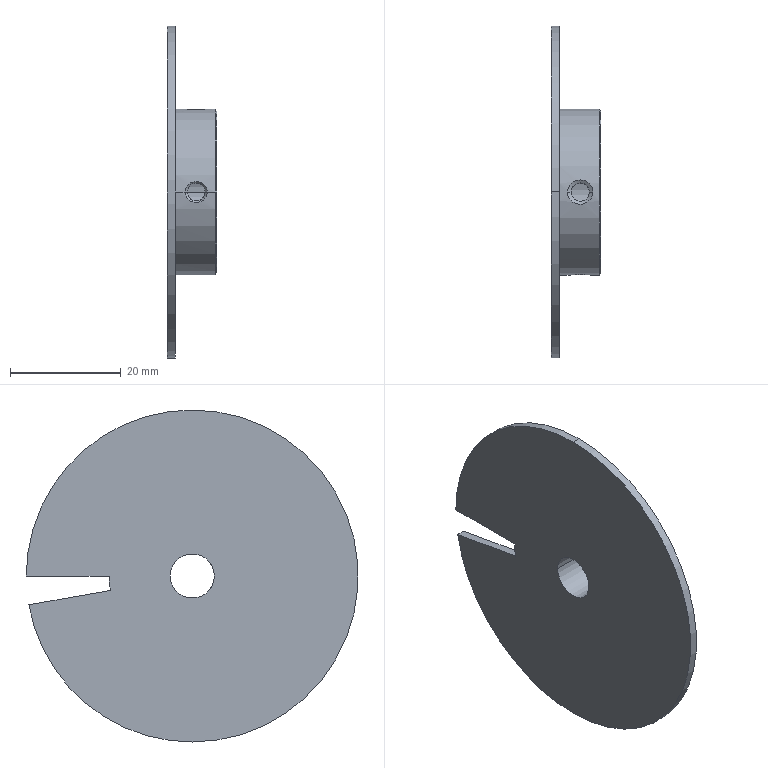Part | NX | 1 solid | 22 faces | box 9 x 60 x 60 mm | volume 8810 mm3 | cylinder 11 | plane 5 | cone 4 | spline 2 | commonest cylinder face diameters 60 x3 3.242 x2 3.3 x2 8 x2 30 x2
STEP:
#1=CARTESIAN_POINT('',(0.,15.,0.));
#2=VERTEX_POINT('',#1);
#3=CARTESIAN_POINT('',(1.5,15.,0.));
#4=VERTEX_POINT('',#3);
#5=CARTESIAN_POINT('',(4.5,15.,0.));
#6=DIRECTION('',(1.,0.,0.));
#7=VECTOR('',#6,1000.);
#8=LINE('',#5,#7);
#9=EDGE_CURVE('',#2,#4,#8,.T.);
#10=ORIENTED_EDGE('',*,*,#9,.T.);
#11=CARTESIAN_POINT('',(8.7,15.,0.));
#12=VERTEX_POINT('',#11);
#13=CARTESIAN_POINT('',(4.5,15.,0.));
#14=DIRECTION('',(1.,0.,0.));
#15=VECTOR('',#14,1000.);
#16=LINE('',#13,#15);
#17=EDGE_CURVE('',#12,#4,#16,.F.);
#18=ORIENTED_EDGE('',*,*,#17,.F.);
#19=CARTESIAN_POINT('',(8.7,-15.,0.));
#20=VERTEX_POINT('',#19);
#21=CARTESIAN_POINT('',(8.7,0.,0.));
#22=DIRECTION('',(-1.,0.,0.));
#23=DIRECTION('',(0.,1.,0.));
#24=AXIS2_PLACEMENT_3D('',#21,#22,#23);
#25=CIRCLE('',#24,15.);
#26=EDGE_CURVE('',#12,#20,#25,.T.);
#27=ORIENTED_EDGE('',*,*,#26,.T.);
#28=CARTESIAN_POINT('',(7.25,-15.,0.));
#29=VERTEX_POINT('',#28);
#30=CARTESIAN_POINT('',(4.5,-15.,0.));
#31=DIRECTION('',(1.,0.,0.));
#32=VECTOR('',#31,1000.);
#33=LINE('',#30,#32);
#34=EDGE_CURVE('',#20,#29,#33,.F.);
#35=ORIENTED_EDGE('',*,*,#34,.T.);
#36=CARTESIAN_POINT('',(3.25,-15.,0.));
#37=VERTEX_POINT('',#36);
#38=CARTESIAN_POINT('',(7.25,-15.,0.));
#39=CARTESIAN_POINT('',(7.25,-15.,-0.5125));
#40=CARTESIAN_POINT('',(6.779,-14.937,-1.503));
#41=CARTESIAN_POINT('',(5.25,-14.854,-2.071));
#42=CARTESIAN_POINT('',(3.721,-14.937,-1.503));
#43=CARTESIAN_POINT('',(3.25,-15.,-0.5127));
#44=CARTESIAN_POINT('',(3.25,-15.,0.));
#45=B_SPLINE_CURVE_WITH_KNOTS('',3,(#38,#39,#40,#41,#42,#43,#44),.UNSPECIFIED.,.F.,.F.,(4,1,1,1,4),(0.,0.25,0.5,0.75,1.),.UNSPECIFIED.);
#46=EDGE_CURVE('',#29,#37,#45,.T.);
#47=ORIENTED_EDGE('',*,*,#46,.T.);
#48=CARTESIAN_POINT('',(1.5,-15.,0.));
#49=VERTEX_POINT('',#48);
#50=CARTESIAN_POINT('',(4.5,-15.,0.));
#51=DIRECTION('',(1.,0.,0.));
#52=VECTOR('',#51,1000.);
#53=LINE('',#50,#52);
#54=EDGE_CURVE('',#49,#37,#53,.T.);
#55=ORIENTED_EDGE('',*,*,#54,.F.);
#56=CARTESIAN_POINT('',(1.5,14.772,-2.605));
#57=VERTEX_POINT('',#56);
#58=CARTESIAN_POINT('',(1.5,0.,0.));
#59=DIRECTION('',(1.,0.,0.));
#60=DIRECTION('',(0.,1.,0.));
#61=AXIS2_PLACEMENT_3D('',#58,#59,#60);
#62=CIRCLE('',#61,15.);
#63=EDGE_CURVE('',#49,#57,#62,.T.);
#64=ORIENTED_EDGE('',*,*,#63,.T.);
#65=CARTESIAN_POINT('',(0.,14.772,-2.605));
#66=VERTEX_POINT('',#65);
#67=CARTESIAN_POINT('',(4.5,14.772,-2.605));
#68=DIRECTION('',(1.,0.,0.));
#69=VECTOR('',#68,1000.);
#70=LINE('',#67,#69);
#71=EDGE_CURVE('',#66,#57,#70,.T.);
#72=ORIENTED_EDGE('',*,*,#71,.F.);
#73=CARTESIAN_POINT('',(0.,0.,0.));
#74=DIRECTION('',(1.,0.,0.));
#75=DIRECTION('',(0.,1.,0.));
#76=AXIS2_PLACEMENT_3D('',#73,#74,#75);
#77=CIRCLE('',#76,15.);
#78=EDGE_CURVE('',#66,#2,#77,.T.);
#79=ORIENTED_EDGE('',*,*,#78,.T.);
#80=EDGE_LOOP('',(#10,#18,#27,#35,#47,#55,#64,#72,#79));
#81=FACE_BOUND('',#80,.T.);
#82=CARTESIAN_POINT('',(4.5,0.,0.));
#83=DIRECTION('',(1.,0.,0.));
#84=DIRECTION('',(0.,1.,0.));
#85=AXIS2_PLACEMENT_3D('',#82,#83,#84);
#86=CYLINDRICAL_SURFACE('',#85,15.);
#87=ADVANCED_FACE('',(#81),#86,.T.);
#88=CARTESIAN_POINT('',(3.629,-14.621,0.));
#89=VERTEX_POINT('',#88);
#90=CARTESIAN_POINT('',(5.25,-14.621,-1.621));
#91=VERTEX_POINT('',#90);
#92=CARTESIAN_POINT('',(5.25,-14.621,0.));
#93=DIRECTION('',(0.,-1.,0.));
#94=DIRECTION('',(0.,0.,1.));
#95=AXIS2_PLACEMENT_3D('',#92,#93,#94);
#96=CIRCLE('',#95,1.621);
#97=EDGE_CURVE('',#89,#91,#96,.T.);
#98=ORIENTED_EDGE('',*,*,#97,.F.);
#99=CARTESIAN_POINT('',(3.439,-14.81,0.));
#100=DIRECTION('',(-0.7071,-0.7071,0.));
#101=VECTOR('',#100,1000.);
#102=LINE('',#99,#101);
#103=EDGE_CURVE('',#37,#89,#102,.F.);
#104=ORIENTED_EDGE('',*,*,#103,.F.);
#105=ORIENTED_EDGE('',*,*,#46,.F.);
#106=CARTESIAN_POINT('',(6.871,-14.621,0.));
#107=VERTEX_POINT('',#106);
#108=CARTESIAN_POINT('',(7.061,-14.81,0.));
#109=DIRECTION('',(0.7071,-0.7071,0.));
#110=VECTOR('',#109,1000.);
#111=LINE('',#108,#110);
#112=EDGE_CURVE('',#29,#107,#111,.F.);
#113=ORIENTED_EDGE('',*,*,#112,.T.);
#114=CARTESIAN_POINT('',(5.25,-14.621,0.));
#115=DIRECTION('',(0.,-1.,0.));
#116=DIRECTION('',(0.,0.,1.));
#117=AXIS2_PLACEMENT_3D('',#114,#115,#116);
#118=CIRCLE('',#117,1.621);
#119=EDGE_CURVE('',#91,#107,#118,.T.);
#120=ORIENTED_EDGE('',*,*,#119,.F.);
#121=EDGE_LOOP('',(#98,#104,#105,#113,#120));
#122=FACE_BOUND('',#121,.T.);
#123=CARTESIAN_POINT('',(5.25,-14.81,0.));
#124=DIRECTION('',(0.,-1.,0.));
#125=DIRECTION('',(-1.,0.,0.));
#126=AXIS2_PLACEMENT_3D('',#123,#124,#125);
#127=CONICAL_SURFACE('',#126,1.81,0.7854);
#128=ADVANCED_FACE('',(#122),#127,.F.);
#129=CARTESIAN_POINT('',(9.,14.7,0.));
#130=VERTEX_POINT('',#129);
#131=CARTESIAN_POINT('',(9.,-14.7,0.));
#132=VERTEX_POINT('',#131);
#133=CARTESIAN_POINT('',(9.,0.,0.));
#134=DIRECTION('',(-1.,0.,0.));
#135=DIRECTION('',(0.,1.,0.));
#136=AXIS2_PLACEMENT_3D('',#133,#134,#135);
#137=CIRCLE('',#136,14.7);
#138=EDGE_CURVE('',#130,#132,#137,.T.);
#139=ORIENTED_EDGE('',*,*,#138,.F.);
#140=CARTESIAN_POINT('',(9.,0.,0.));
#141=DIRECTION('',(-1.,0.,0.));
#142=DIRECTION('',(0.,1.,0.));
#143=AXIS2_PLACEMENT_3D('',#140,#141,#142);
#144=CIRCLE('',#143,14.7);
#145=EDGE_CURVE('',#132,#130,#144,.T.);
#146=ORIENTED_EDGE('',*,*,#145,.F.);
#147=EDGE_LOOP('',(#139,#146));
#148=FACE_BOUND('',#147,.T.);
#149=CARTESIAN_POINT('',(9.,4.,0.));
#150=VERTEX_POINT('',#149);
#151=CARTESIAN_POINT('',(9.,-4.,0.));
#152=VERTEX_POINT('',#151);
#153=CARTESIAN_POINT('',(9.,0.,0.));
#154=DIRECTION('',(1.,0.,0.));
#155=DIRECTION('',(0.,1.,0.));
#156=AXIS2_PLACEMENT_3D('',#153,#154,#155);
#157=CIRCLE('',#156,4.);
#158=EDGE_CURVE('',#150,#152,#157,.T.);
#159=ORIENTED_EDGE('',*,*,#158,.F.);
#160=CARTESIAN_POINT('',(9.,0.,0.));
#161=DIRECTION('',(1.,0.,0.));
#162=DIRECTION('',(0.,1.,0.));
#163=AXIS2_PLACEMENT_3D('',#160,#161,#162);
#164=CIRCLE('',#163,4.);
#165=EDGE_CURVE('',#152,#150,#164,.T.);
#166=ORIENTED_EDGE('',*,*,#165,.F.);
#167=EDGE_LOOP('',(#159,#166));
#168=FACE_BOUND('',#167,.T.);
#169=CARTESIAN_POINT('',(9.,7.5,0.));
#170=DIRECTION('',(1.,0.,0.));
#171=DIRECTION('',(0.,1.,0.));
#172=AXIS2_PLACEMENT_3D('',#169,#170,#171);
#173=PLANE('',#172);
#174=ADVANCED_FACE('',(#148,#168),#173,.T.);
#175=CARTESIAN_POINT('',(0.,4.,0.));
#176=VERTEX_POINT('',#175);
#177=CARTESIAN_POINT('',(0.,-4.,0.));
#178=VERTEX_POINT('',#177);
#179=CARTESIAN_POINT('',(0.,0.,0.));
#180=DIRECTION('',(1.,0.,0.));
#181=DIRECTION('',(0.,1.,0.));
#182=AXIS2_PLACEMENT_3D('',#179,#180,#181);
#183=CIRCLE('',#182,4.);
#184=EDGE_CURVE('',#176,#178,#183,.T.);
#185=ORIENTED_EDGE('',*,*,#184,.F.);
#186=CARTESIAN_POINT('',(4.5,4.,0.));
#187=DIRECTION('',(1.,0.,0.));
#188=VECTOR('',#187,1000.);
#189=LINE('',#186,#188);
#190=EDGE_CURVE('',#176,#150,#189,.T.);
#191=ORIENTED_EDGE('',*,*,#190,.T.);
#192=ORIENTED_EDGE('',*,*,#158,.T.);
#193=CARTESIAN_POINT('',(6.871,-4.,0.));
#194=VERTEX_POINT('',#193);
#195=CARTESIAN_POINT('',(4.5,-4.,0.));
#196=DIRECTION('',(1.,0.,0.));
#197=VECTOR('',#196,1000.);
#198=LINE('',#195,#197);
#199=EDGE_CURVE('',#194,#152,#198,.T.);
#200=ORIENTED_EDGE('',*,*,#199,.F.);
#201=CARTESIAN_POINT('',(5.25,-3.657,1.621));
#202=VERTEX_POINT('',#201);
#203=CARTESIAN_POINT('',(6.871,-4.,0.));
#204=CARTESIAN_POINT('',(6.871,-4.,0.8631));
#205=CARTESIAN_POINT('',(6.111,-3.657,1.621));
#206=CARTESIAN_POINT('',(5.25,-3.657,1.621));
#207=B_SPLINE_CURVE_WITH_KNOTS('',3,(#203,#204,#205,#206),.UNSPECIFIED.,.F.,.F.,(4,4),(0.,1.),.UNSPECIFIED.);
#208=EDGE_CURVE('',#202,#194,#207,.F.);
#209=ORIENTED_EDGE('',*,*,#208,.F.);
#210=CARTESIAN_POINT('',(3.629,-4.,0.));
#211=VERTEX_POINT('',#210);
#212=CARTESIAN_POINT('',(5.25,-3.657,1.621));
#213=CARTESIAN_POINT('',(4.837,-3.657,1.621));
#214=CARTESIAN_POINT('',(3.975,-3.836,1.267));
#215=CARTESIAN_POINT('',(3.629,-4.,0.4316));
#216=CARTESIAN_POINT('',(3.629,-4.,0.));
#217=B_SPLINE_CURVE_WITH_KNOTS('',3,(#212,#213,#214,#215,#216),.UNSPECIFIED.,.F.,.F.,(4,1,4),(0.,0.5,1.),.UNSPECIFIED.);
#218=EDGE_CURVE('',#211,#202,#217,.F.);
#219=ORIENTED_EDGE('',*,*,#218,.F.);
#220=CARTESIAN_POINT('',(4.5,-4.,0.));
#221=DIRECTION('',(1.,0.,0.));
#222=VECTOR('',#221,1000.);
#223=LINE('',#220,#222);
#224=EDGE_CURVE('',#178,#211,#223,.T.);
#225=ORIENTED_EDGE('',*,*,#224,.F.);
#226=EDGE_LOOP('',(#185,#191,#192,#200,#209,#219,#225));
#227=FACE_BOUND('',#226,.T.);
#228=CARTESIAN_POINT('',(5.25,-1.65,3.644));
#229=VERTEX_POINT('',#228);
#230=CARTESIAN_POINT('',(5.25,1.65,3.644));
#231=VERTEX_POINT('',#230);
#232=CARTESIAN_POINT('',(5.25,-1.65,3.644));
#233=CARTESIAN_POINT('',(5.688,-1.65,3.644));
#234=CARTESIAN_POINT('',(6.538,-1.294,3.83));
#235=CARTESIAN_POINT('',(7.081,-0.00007192,4.085));
#236=CARTESIAN_POINT('',(6.538,1.294,3.83));
#237=CARTESIAN_POINT('',(5.687,1.65,3.644));
#238=CARTESIAN_POINT('',(5.25,1.65,3.644));
#239=B_SPLINE_CURVE_WITH_KNOTS('',3,(#232,#233,#234,#235,#236,#237,#238),.UNSPECIFIED.,.F.,.F.,(4,1,1,1,4),(0.,0.25,0.5,0.75,1.),.UNSPECIFIED.);
#240=EDGE_CURVE('',#229,#231,#239,.T.);
#241=ORIENTED_EDGE('',*,*,#240,.T.);
#242=CARTESIAN_POINT('',(5.25,1.65,3.644));
#243=CARTESIAN_POINT('',(4.813,1.65,3.644));
#244=CARTESIAN_POINT('',(3.961,1.294,3.83));
#245=CARTESIAN_POINT('',(3.419,-0.00003824,4.085));
#246=CARTESIAN_POINT('',(3.961,-1.294,3.83));
#247=CARTESIAN_POINT('',(4.813,-1.65,3.644));
#248=CARTESIAN_POINT('',(5.25,-1.65,3.644));
#249=B_SPLINE_CURVE_WITH_KNOTS('',3,(#242,#243,#244,#245,#246,#247,#248),.UNSPECIFIED.,.F.,.F.,(4,1,1,1,4),(0.,0.25,0.5,0.75,1.),.UNSPECIFIED.);
#250=EDGE_CURVE('',#231,#229,#249,.T.);
#251=ORIENTED_EDGE('',*,*,#250,.T.);
#252=EDGE_LOOP('',(#241,#251));
#253=FACE_BOUND('',#252,.T.);
#254=CARTESIAN_POINT('',(4.5,0.,0.));
#255=DIRECTION('',(1.,0.,0.));
#256=DIRECTION('',(0.,1.,0.));
#257=AXIS2_PLACEMENT_3D('',#254,#255,#256);
#258=CYLINDRICAL_SURFACE('',#257,4.);
#259=ADVANCED_FACE('',(#227,#253),#258,.F.);
#260=ORIENTED_EDGE('',*,*,#97,.T.);
#261=CARTESIAN_POINT('',(5.25,-3.657,-1.621));
#262=VERTEX_POINT('',#261);
#263=CARTESIAN_POINT('',(5.25,-9.06,-1.621));
#264=DIRECTION('',(0.,1.,0.));
#265=VECTOR('',#264,1000.);
#266=LINE('',#263,#265);
#267=EDGE_CURVE('',#262,#91,#266,.F.);
#268=ORIENTED_EDGE('',*,*,#267,.F.);
#269=CARTESIAN_POINT('',(5.25,-3.657,-1.621));
#270=CARTESIAN_POINT('',(5.05,-3.657,-1.621));
#271=CARTESIAN_POINT('',(4.729,-3.682,-1.57));
#272=CARTESIAN_POINT('',(4.364,-3.762,-1.361));
#273=CARTESIAN_POINT('',(4.261,-3.788,-1.287));
#274=CARTESIAN_POINT('',(4.044,-3.848,-1.102));
#275=CARTESIAN_POINT('',(3.861,-3.91,-0.8502));
#276=CARTESIAN_POINT('',(3.715,-3.966,-0.5735));
#277=CARTESIAN_POINT('',(3.629,-4.,-0.2033));
#278=CARTESIAN_POINT('',(3.629,-4.,0.));
#279=B_SPLINE_CURVE_WITH_KNOTS('',3,(#269,#270,#271,#272,#273,#274,#275,#276,#277,#278),.UNSPECIFIED.,.F.,.F.,(4,1,1,1,1,1,1,4),(0.,0.25,0.375,0.4375,0.5,0.625,0.75,1.),.UNSPECIFIED.);
#280=EDGE_CURVE('',#262,#211,#279,.T.);
#281=ORIENTED_EDGE('',*,*,#280,.T.);
#282=ORIENTED_EDGE('',*,*,#218,.T.);
#283=CARTESIAN_POINT('',(5.25,-14.621,1.621));
#284=VERTEX_POINT('',#283);
#285=CARTESIAN_POINT('',(5.25,-9.06,1.621));
#286=DIRECTION('',(0.,1.,0.));
#287=VECTOR('',#286,1000.);
#288=LINE('',#285,#287);
#289=EDGE_CURVE('',#202,#284,#288,.F.);
#290=ORIENTED_EDGE('',*,*,#289,.T.);
#291=CARTESIAN_POINT('',(5.25,-14.621,0.));
#292=DIRECTION('',(0.,-1.,0.));
#293=DIRECTION('',(0.,0.,1.));
#294=AXIS2_PLACEMENT_3D('',#291,#292,#293);
#295=CIRCLE('',#294,1.621);
#296=EDGE_CURVE('',#284,#89,#295,.T.);
#297=ORIENTED_EDGE('',*,*,#296,.T.);
#298=EDGE_LOOP('',(#260,#268,#281,#282,#290,#297));
#299=FACE_BOUND('',#298,.T.);
#300=CARTESIAN_POINT('',(5.25,-9.06,0.));
#301=DIRECTION('',(0.,1.,0.));
#302=DIRECTION('',(0.,0.,1.));
#303=AXIS2_PLACEMENT_3D('',#300,#301,#302);
#304=CYLINDRICAL_SURFACE('',#303,1.621);
#305=ADVANCED_FACE('',(#299),#304,.F.);
#306=CARTESIAN_POINT('',(0.,30.,0.));
#307=VERTEX_POINT('',#306);
#308=CARTESIAN_POINT('',(0.,30.,0.));
#309=DIRECTION('',(0.,-1.,0.));
#310=VECTOR('',#309,1000.);
#311=LINE('',#308,#310);
#312=EDGE_CURVE('',#307,#2,#311,.T.);
#313=ORIENTED_EDGE('',*,*,#312,.T.);
#314=ORIENTED_EDGE('',*,*,#78,.F.);
#315=CARTESIAN_POINT('',(0.,29.544,-5.209));
#316=VERTEX_POINT('',#315);
#317=CARTESIAN_POINT('',(0.,29.544,-5.209));
#318=DIRECTION('',(0.,-0.9848,0.1736));
#319=VECTOR('',#318,1000.);
#320=LINE('',#317,#319);
#321=EDGE_CURVE('',#316,#66,#320,.T.);
#322=ORIENTED_EDGE('',*,*,#321,.F.);
#323=CARTESIAN_POINT('',(0.,0.,-30.));
#324=VERTEX_POINT('',#323);
#325=CARTESIAN_POINT('',(0.,0.,0.));
#326=DIRECTION('',(1.,0.,0.));
#327=DIRECTION('',(0.,0.,-1.));
#328=AXIS2_PLACEMENT_3D('',#325,#326,#327);
#329=CIRCLE('',#328,30.);
#330=EDGE_CURVE('',#324,#316,#329,.T.);
#331=ORIENTED_EDGE('',*,*,#330,.F.);
#332=CARTESIAN_POINT('',(0.,0.,30.));
#333=VERTEX_POINT('',#332);
#334=CARTESIAN_POINT('',(0.,0.,0.));
#335=DIRECTION('',(1.,0.,0.));
#336=DIRECTION('',(0.,0.,-1.));
#337=AXIS2_PLACEMENT_3D('',#334,#335,#336);
#338=CIRCLE('',#337,30.);
#339=EDGE_CURVE('',#333,#324,#338,.T.);
#340=ORIENTED_EDGE('',*,*,#339,.F.);
#341=CARTESIAN_POINT('',(0.,0.,0.));
#342=DIRECTION('',(1.,0.,0.));
#343=DIRECTION('',(0.,0.,-1.));
#344=AXIS2_PLACEMENT_3D('',#341,#342,#343);
#345=CIRCLE('',#344,30.);
#346=EDGE_CURVE('',#307,#333,#345,.T.);
#347=ORIENTED_EDGE('',*,*,#346,.F.);
#348=EDGE_LOOP('',(#313,#314,#322,#331,#340,#347));
#349=FACE_BOUND('',#348,.T.);
#350=ORIENTED_EDGE('',*,*,#184,.T.);
#351=CARTESIAN_POINT('',(0.,0.,0.));
#352=DIRECTION('',(1.,0.,0.));
#353=DIRECTION('',(0.,1.,0.));
#354=AXIS2_PLACEMENT_3D('',#351,#352,#353);
#355=CIRCLE('',#354,4.);
#356=EDGE_CURVE('',#178,#176,#355,.T.);
#357=ORIENTED_EDGE('',*,*,#356,.T.);
#358=EDGE_LOOP('',(#350,#357));
#359=FACE_BOUND('',#358,.T.);
#360=CARTESIAN_POINT('',(0.,7.5,0.));
#361=DIRECTION('',(-1.,0.,0.));
#362=DIRECTION('',(0.,0.,1.));
#363=AXIS2_PLACEMENT_3D('',#360,#361,#362);
#364=PLANE('',#363);
#365=ADVANCED_FACE('',(#349,#359),#364,.T.);
#366=CARTESIAN_POINT('',(1.5,30.,0.));
#367=VERTEX_POINT('',#366);
#368=CARTESIAN_POINT('',(0.,30.,0.));
#369=DIRECTION('',(1.,0.,0.));
#370=VECTOR('',#369,1000.);
#371=LINE('',#368,#370);
#372=EDGE_CURVE('',#307,#367,#371,.T.);
#373=ORIENTED_EDGE('',*,*,#372,.T.);
#374=CARTESIAN_POINT('',(1.5,15.,0.));
#375=DIRECTION('',(0.,1.,0.));
#376=VECTOR('',#375,1000.);
#377=LINE('',#374,#376);
#378=EDGE_CURVE('',#4,#367,#377,.T.);
#379=ORIENTED_EDGE('',*,*,#378,.F.);
#380=ORIENTED_EDGE('',*,*,#9,.F.);
#381=ORIENTED_EDGE('',*,*,#312,.F.);
#382=EDGE_LOOP('',(#373,#379,#380,#381));
#383=FACE_BOUND('',#382,.T.);
#384=CARTESIAN_POINT('',(0.,15.,0.));
#385=DIRECTION('',(0.,0.,1.));
#386=DIRECTION('',(1.,0.,0.));
#387=AXIS2_PLACEMENT_3D('',#384,#385,#386);
#388=PLANE('',#387);
#389=ADVANCED_FACE('',(#383),#388,.F.);
#390=CARTESIAN_POINT('',(1.5,0.,30.));
#391=VERTEX_POINT('',#390);
#392=CARTESIAN_POINT('',(0.,0.,30.));
#393=DIRECTION('',(-1.,0.,0.));
#394=VECTOR('',#393,1000.);
#395=LINE('',#392,#394);
#396=EDGE_CURVE('',#391,#333,#395,.T.);
#397=ORIENTED_EDGE('',*,*,#396,.F.);
#398=CARTESIAN_POINT('',(1.5,0.,0.));
#399=DIRECTION('',(-1.,0.,0.));
#400=DIRECTION('',(0.,0.,1.));
#401=AXIS2_PLACEMENT_3D('',#398,#399,#400);
#402=CIRCLE('',#401,30.);
#403=EDGE_CURVE('',#391,#367,#402,.T.);
#404=ORIENTED_EDGE('',*,*,#403,.T.);
#405=ORIENTED_EDGE('',*,*,#372,.F.);
#406=ORIENTED_EDGE('',*,*,#346,.T.);
#407=EDGE_LOOP('',(#397,#404,#405,#406));
#408=FACE_BOUND('',#407,.T.);
#409=CARTESIAN_POINT('',(0.,0.,0.));
#410=DIRECTION('',(-1.,0.,0.));
#411=DIRECTION('',(0.,0.,-1.));
#412=AXIS2_PLACEMENT_3D('',#409,#410,#411);
#413=CYLINDRICAL_SURFACE('',#412,30.);
#414=ADVANCED_FACE('',(#408),#413,.T.);
#415=ORIENTED_EDGE('',*,*,#378,.T.);
#416=ORIENTED_EDGE('',*,*,#403,.F.);
#417=CARTESIAN_POINT('',(1.5,0.,-30.));
#418=VERTEX_POINT('',#417);
#419=CARTESIAN_POINT('',(1.5,0.,0.));
#420=DIRECTION('',(-1.,0.,0.));
#421=DIRECTION('',(0.,0.,1.));
#422=AXIS2_PLACEMENT_3D('',#419,#420,#421);
#423=CIRCLE('',#422,30.);
#424=EDGE_CURVE('',#418,#391,#423,.T.);
#425=ORIENTED_EDGE('',*,*,#424,.F.);
#426=CARTESIAN_POINT('',(1.5,29.544,-5.209));
#427=VERTEX_POINT('',#426);
#428=CARTESIAN_POINT('',(1.5,0.,0.));
#429=DIRECTION('',(-1.,0.,0.));
#430=DIRECTION('',(0.,0.,1.));
#431=AXIS2_PLACEMENT_3D('',#428,#429,#430);
#432=CIRCLE('',#431,30.);
#433=EDGE_CURVE('',#427,#418,#432,.T.);
#434=ORIENTED_EDGE('',*,*,#433,.F.);
#435=CARTESIAN_POINT('',(1.5,14.772,-2.605));
#436=DIRECTION('',(0.,0.9848,-0.1736));
#437=VECTOR('',#436,1000.);
#438=LINE('',#435,#437);
#439=EDGE_CURVE('',#57,#427,#438,.T.);
#440=ORIENTED_EDGE('',*,*,#439,.F.);
#441=ORIENTED_EDGE('',*,*,#63,.F.);
#442=CARTESIAN_POINT('',(1.5,0.,0.));
#443=DIRECTION('',(1.,0.,0.));
#444=DIRECTION('',(0.,1.,0.));
#445=AXIS2_PLACEMENT_3D('',#442,#443,#444);
#446=CIRCLE('',#445,15.);
#447=EDGE_CURVE('',#4,#49,#446,.T.);
#448=ORIENTED_EDGE('',*,*,#447,.F.);
#449=EDGE_LOOP('',(#415,#416,#425,#434,#440,#441,#448));
#450=FACE_BOUND('',#449,.T.);
#451=CARTESIAN_POINT('',(1.5,0.,0.));
#452=DIRECTION('',(1.,0.,0.));
#453=DIRECTION('',(0.,1.,0.));
#454=AXIS2_PLACEMENT_3D('',#451,#452,#453);
#455=PLANE('',#454);
#456=ADVANCED_FACE('',(#450),#455,.T.);
#457=CARTESIAN_POINT('',(1.5,29.544,-5.209));
#458=DIRECTION('',(-1.,0.,0.));
#459=VECTOR('',#458,1000.);
#460=LINE('',#457,#459);
#461=EDGE_CURVE('',#427,#316,#460,.T.);
#462=ORIENTED_EDGE('',*,*,#461,.T.);
#463=ORIENTED_EDGE('',*,*,#321,.T.);
#464=ORIENTED_EDGE('',*,*,#71,.T.);
#465=ORIENTED_EDGE('',*,*,#439,.T.);
#466=EDGE_LOOP('',(#462,#463,#464,#465));
#467=FACE_BOUND('',#466,.T.);
#468=CARTESIAN_POINT('',(0.,31.099,-5.484));
#469=DIRECTION('',(0.,-0.1736,-0.9848));
#470=DIRECTION('',(0.,-0.9848,0.1736));
#471=AXIS2_PLACEMENT_3D('',#468,#469,#470);
#472=PLANE('',#471);
#473=ADVANCED_FACE('',(#467),#472,.F.);
#474=CARTESIAN_POINT('',(5.25,-1.65,14.525));
#475=VERTEX_POINT('',#474);
#476=CARTESIAN_POINT('',(6.9,0.007829,14.616));
#477=VERTEX_POINT('',#476);
#478=CARTESIAN_POINT('',(5.25,-1.65,14.525));
#479=CARTESIAN_POINT('',(5.461,-1.65,14.525));
#480=CARTESIAN_POINT('',(5.848,-1.555,14.535));
#481=CARTESIAN_POINT('',(6.119,-1.413,14.549));
#482=CARTESIAN_POINT('',(6.449,-1.164,14.571));
#483=CARTESIAN_POINT('',(6.683,-0.8348,14.593));
#484=CARTESIAN_POINT('',(6.817,-0.5655,14.607));
#485=CARTESIAN_POINT('',(6.901,-0.1951,14.616));
#486=CARTESIAN_POINT('',(6.9,0.007828,14.616));
#487=B_SPLINE_CURVE_WITH_KNOTS('',3,(#478,#479,#480,#481,#482,#483,#484,#485,#486),.UNSPECIFIED.,.F.,.F.,(4,1,1,1,1,1,4),(0.,0.25,0.375,0.5,0.625,0.75,1.),.UNSPECIFIED.);
#488=EDGE_CURVE('',#475,#477,#487,.T.);
#489=ORIENTED_EDGE('',*,*,#488,.T.);
#490=CARTESIAN_POINT('',(5.25,1.65,14.525));
#491=VERTEX_POINT('',#490);
#492=CARTESIAN_POINT('',(6.9,0.007828,14.616));
#493=CARTESIAN_POINT('',(6.899,0.2061,14.616));
#494=CARTESIAN_POINT('',(6.812,0.5787,14.606));
#495=CARTESIAN_POINT('',(6.677,0.8437,14.592));
#496=CARTESIAN_POINT('',(6.443,1.17,14.571));
#497=CARTESIAN_POINT('',(6.11,1.418,14.549));
#498=CARTESIAN_POINT('',(5.847,1.555,14.535));
#499=CARTESIAN_POINT('',(5.46,1.65,14.525));
#500=CARTESIAN_POINT('',(5.25,1.65,14.525));
#501=B_SPLINE_CURVE_WITH_KNOTS('',3,(#492,#493,#494,#495,#496,#497,#498,#499,#500),.UNSPECIFIED.,.F.,.F.,(4,1,1,1,1,1,4),(0.,0.25,0.375,0.5,0.625,0.75,1.),.UNSPECIFIED.);
#502=EDGE_CURVE('',#477,#491,#501,.T.);
#503=ORIENTED_EDGE('',*,*,#502,.T.);
#504=CARTESIAN_POINT('',(5.25,1.65,15.));
#505=DIRECTION('',(0.,0.,1.));
#506=VECTOR('',#505,1000.);
#507=LINE('',#504,#506);
#508=EDGE_CURVE('',#231,#491,#507,.T.);
#509=ORIENTED_EDGE('',*,*,#508,.F.);
#510=ORIENTED_EDGE('',*,*,#240,.F.);
#511=CARTESIAN_POINT('',(5.25,-1.65,15.));
#512=DIRECTION('',(0.,0.,1.));
#513=VECTOR('',#512,1000.);
#514=LINE('',#511,#513);
#515=EDGE_CURVE('',#229,#475,#514,.T.);
#516=ORIENTED_EDGE('',*,*,#515,.T.);
#517=EDGE_LOOP('',(#489,#503,#509,#510,#516));
#518=FACE_BOUND('',#517,.T.);
#519=CARTESIAN_POINT('',(5.25,0.,15.));
#520=DIRECTION('',(0.,0.,1.));
#521=DIRECTION('',(0.,1.,0.));
#522=AXIS2_PLACEMENT_3D('',#519,#520,#521);
#523=CYLINDRICAL_SURFACE('',#522,1.65);
#524=ADVANCED_FACE('',(#518),#523,.F.);
#525=CARTESIAN_POINT('',(7.564,0.01193,15.));
#526=VERTEX_POINT('',#525);
#527=CARTESIAN_POINT('',(2.935,-0.01286,15.));
#528=VERTEX_POINT('',#527);
#529=CARTESIAN_POINT('',(2.935,-0.01286,15.));
#530=CARTESIAN_POINT('',(2.932,0.5932,15.001));
#531=CARTESIAN_POINT('',(3.497,1.762,14.914));
#532=CARTESIAN_POINT('',(5.24,2.405,14.802));
#533=CARTESIAN_POINT('',(6.98,1.78,14.911));
#534=CARTESIAN_POINT('',(7.562,0.6172,15.));
#535=CARTESIAN_POINT('',(7.564,0.01193,15.));
#536=B_SPLINE_CURVE_WITH_KNOTS('',3,(#529,#530,#531,#532,#533,#534,#535),.UNSPECIFIED.,.F.,.F.,(4,1,1,1,4),(0.,0.25,0.5,0.75,1.),.UNSPECIFIED.);
#537=EDGE_CURVE('',#526,#528,#536,.F.);
#538=ORIENTED_EDGE('',*,*,#537,.T.);
#539=CARTESIAN_POINT('',(3.6,-0.008997,14.616));
#540=VERTEX_POINT('',#539);
#541=CARTESIAN_POINT('',(3.6,-0.008997,14.616));
#542=CARTESIAN_POINT('',(2.935,-0.01286,15.));
#543=B_SPLINE_CURVE_WITH_KNOTS('',1,(#541,#542),.UNSPECIFIED.,.F.,.F.,(2,2),(0.,1.),.UNSPECIFIED.);
#544=EDGE_CURVE('',#540,#528,#543,.T.);
#545=ORIENTED_EDGE('',*,*,#544,.F.);
#546=CARTESIAN_POINT('',(5.25,1.65,14.525));
#547=CARTESIAN_POINT('',(5.045,1.65,14.525));
#548=CARTESIAN_POINT('',(4.65,1.555,14.535));
#549=CARTESIAN_POINT('',(4.383,1.414,14.549));
#550=CARTESIAN_POINT('',(4.051,1.164,14.571));
#551=CARTESIAN_POINT('',(3.816,0.8324,14.593));
#552=CARTESIAN_POINT('',(3.683,0.5655,14.607));
#553=CARTESIAN_POINT('',(3.599,0.19,14.616));
#554=CARTESIAN_POINT('',(3.6,-0.008997,14.616));
#555=B_SPLINE_CURVE_WITH_KNOTS('',3,(#546,#547,#548,#549,#550,#551,#552,#553,#554),.UNSPECIFIED.,.F.,.F.,(4,1,1,1,1,1,4),(0.,0.25,0.375,0.5,0.625,0.75,1.),.UNSPECIFIED.);
#556=EDGE_CURVE('',#491,#540,#555,.T.);
#557=ORIENTED_EDGE('',*,*,#556,.F.);
#558=ORIENTED_EDGE('',*,*,#502,.F.);
#559=CARTESIAN_POINT('',(6.9,0.007829,14.616));
#560=CARTESIAN_POINT('',(7.564,0.01193,15.));
#561=B_SPLINE_CURVE_WITH_KNOTS('',1,(#559,#560),.UNSPECIFIED.,.F.,.F.,(2,2),(0.,1.),.UNSPECIFIED.);
#562=EDGE_CURVE('',#477,#526,#561,.T.);
#563=ORIENTED_EDGE('',*,*,#562,.T.);
#564=EDGE_LOOP('',(#538,#545,#557,#558,#563));
#565=FACE_BOUND('',#564,.T.);
#566=CARTESIAN_POINT('',(6.9,0.007829,14.616));
#567=CARTESIAN_POINT('',(7.564,0.01193,15.));
#568=CARTESIAN_POINT('',(6.9,0.09255,14.616));
#569=CARTESIAN_POINT('',(7.564,0.1331,15.));
#570=CARTESIAN_POINT('',(6.893,0.1775,14.615));
#571=CARTESIAN_POINT('',(7.553,0.2544,14.998));
#572=CARTESIAN_POINT('',(6.836,0.5282,14.609));
#573=CARTESIAN_POINT('',(7.461,0.7494,14.986));
#574=CARTESIAN_POINT('',(6.73,0.7792,14.597));
#575=CARTESIAN_POINT('',(7.288,1.098,14.963));
#576=CARTESIAN_POINT('',(6.399,1.215,14.568));
#577=CARTESIAN_POINT('',(6.796,1.669,14.91));
#578=CARTESIAN_POINT('',(6.179,1.392,14.551));
#579=CARTESIAN_POINT('',(6.486,1.885,14.882));
#580=CARTESIAN_POINT('',(5.671,1.619,14.529));
#581=CARTESIAN_POINT('',(5.798,2.159,14.844));
#582=CARTESIAN_POINT('',(5.388,1.668,14.523));
#583=CARTESIAN_POINT('',(5.433,2.214,14.836));
#584=CARTESIAN_POINT('',(4.831,1.62,14.528));
#585=CARTESIAN_POINT('',(4.699,2.158,14.844));
#586=CARTESIAN_POINT('',(4.561,1.525,14.539));
#587=CARTESIAN_POINT('',(4.344,2.048,14.861));
#588=CARTESIAN_POINT('',(4.101,1.216,14.567));
#589=CARTESIAN_POINT('',(3.705,1.667,14.908));
#590=CARTESIAN_POINT('',(3.916,1.009,14.583));
#591=CARTESIAN_POINT('',(3.432,1.402,14.938));
#592=CARTESIAN_POINT('',(3.664,0.5294,14.608));
#593=CARTESIAN_POINT('',(3.043,0.7555,14.984));
#594=CARTESIAN_POINT('',(3.6,0.2673,14.616));
#595=CARTESIAN_POINT('',(2.935,0.3809,15.));
#596=CARTESIAN_POINT('',(3.6,-0.003047,14.616));
#597=CARTESIAN_POINT('',(2.935,-0.004342,15.));
#598=CARTESIAN_POINT('',(3.6,-0.00602,14.616));
#599=CARTESIAN_POINT('',(2.935,-0.008604,15.));
#600=CARTESIAN_POINT('',(3.6,-0.008997,14.616));
#601=CARTESIAN_POINT('',(2.935,-0.01286,15.));
#602=B_SPLINE_SURFACE_WITH_KNOTS('',3,1,((#566,#567),(#568,#569),(#570,#571),(#572,#573),(#574,#575),(#576,#577),(#578,#579),(#580,#581),(#582,#583),(#584,#585),(#586,#587),(#588,#589),(#590,#591),(#592,#593),(#594,#595),(#596,#597),(#598,#599),(#600,#601)),.RULED_SURF.,.F.,.F.,.F.,(4,2,2,2,2,2,2,2,4),(2,2),(6.186,6.497,7.474,8.456,9.432,10.412,11.389,12.36,12.371),(0.,1.),.UNSPECIFIED.);
#603=ADVANCED_FACE('',(#565),#602,.F.);
#604=ORIENTED_EDGE('',*,*,#138,.T.);
#605=CARTESIAN_POINT('',(9.,-14.7,0.));
#606=DIRECTION('',(-0.7071,-0.7071,0.));
#607=VECTOR('',#606,1000.);
#608=LINE('',#605,#607);
#609=EDGE_CURVE('',#20,#132,#608,.F.);
#610=ORIENTED_EDGE('',*,*,#609,.F.);
#611=ORIENTED_EDGE('',*,*,#26,.F.);
#612=CARTESIAN_POINT('',(9.,14.7,0.));
#613=DIRECTION('',(-0.7071,0.7071,0.));
#614=VECTOR('',#613,1000.);
#615=LINE('',#612,#614);
#616=EDGE_CURVE('',#12,#130,#615,.F.);
#617=ORIENTED_EDGE('',*,*,#616,.T.);
#618=EDGE_LOOP('',(#604,#610,#611,#617));
#619=FACE_BOUND('',#618,.T.);
#620=CARTESIAN_POINT('',(9.,0.,0.));
#621=DIRECTION('',(-1.,0.,0.));
#622=DIRECTION('',(0.,1.,0.));
#623=AXIS2_PLACEMENT_3D('',#620,#621,#622);
#624=CONICAL_SURFACE('',#623,14.7,0.7854);
#625=ADVANCED_FACE('',(#619),#624,.T.);
#626=ORIENTED_EDGE('',*,*,#208,.T.);
#627=CARTESIAN_POINT('',(6.871,-4.,0.));
#628=CARTESIAN_POINT('',(6.871,-4.,-0.2032));
#629=CARTESIAN_POINT('',(6.81,-3.974,-0.5349));
#630=CARTESIAN_POINT('',(6.597,-3.896,-0.9146));
#631=CARTESIAN_POINT('',(6.462,-3.85,-1.093));
#632=CARTESIAN_POINT('',(6.237,-3.787,-1.289));
#633=CARTESIAN_POINT('',(6.137,-3.762,-1.359));
#634=CARTESIAN_POINT('',(5.77,-3.682,-1.571));
#635=CARTESIAN_POINT('',(5.45,-3.657,-1.621));
#636=CARTESIAN_POINT('',(5.25,-3.657,-1.621));
#637=B_SPLINE_CURVE_WITH_KNOTS('',3,(#627,#628,#629,#630,#631,#632,#633,#634,#635,#636),.UNSPECIFIED.,.F.,.F.,(4,1,1,1,1,1,1,4),(0.,0.25,0.375,0.5,0.5625,0.625,0.75,1.),.UNSPECIFIED.);
#638=EDGE_CURVE('',#194,#262,#637,.T.);
#639=ORIENTED_EDGE('',*,*,#638,.T.);
#640=ORIENTED_EDGE('',*,*,#267,.T.);
#641=ORIENTED_EDGE('',*,*,#119,.T.);
#642=CARTESIAN_POINT('',(5.25,-14.621,0.));
#643=DIRECTION('',(0.,-1.,0.));
#644=DIRECTION('',(0.,0.,1.));
#645=AXIS2_PLACEMENT_3D('',#642,#643,#644);
#646=CIRCLE('',#645,1.621);
#647=EDGE_CURVE('',#107,#284,#646,.T.);
#648=ORIENTED_EDGE('',*,*,#647,.T.);
#649=ORIENTED_EDGE('',*,*,#289,.F.);
#650=EDGE_LOOP('',(#626,#639,#640,#641,#648,#649));
#651=FACE_BOUND('',#650,.T.);
#652=CARTESIAN_POINT('',(5.25,-9.06,0.));
#653=DIRECTION('',(0.,1.,0.));
#654=DIRECTION('',(0.,0.,1.));
#655=AXIS2_PLACEMENT_3D('',#652,#653,#654);
#656=CYLINDRICAL_SURFACE('',#655,1.621);
#657=ADVANCED_FACE('',(#651),#656,.F.);
#658=ORIENTED_EDGE('',*,*,#508,.T.);
#659=ORIENTED_EDGE('',*,*,#556,.T.);
#660=CARTESIAN_POINT('',(3.6,-0.008997,14.616));
#661=CARTESIAN_POINT('',(3.601,-0.209,14.616));
#662=CARTESIAN_POINT('',(3.69,-0.5823,14.606));
#663=CARTESIAN_POINT('',(3.822,-0.8435,14.592));
#664=CARTESIAN_POINT('',(4.059,-1.172,14.571));
#665=CARTESIAN_POINT('',(4.385,-1.415,14.549));
#666=CARTESIAN_POINT('',(4.658,-1.558,14.535));
#667=CARTESIAN_POINT('',(5.04,-1.65,14.525));
#668=CARTESIAN_POINT('',(5.25,-1.65,14.525));
#669=B_SPLINE_CURVE_WITH_KNOTS('',3,(#660,#661,#662,#663,#664,#665,#666,#667,#668),.UNSPECIFIED.,.F.,.F.,(4,1,1,1,1,1,4),(0.,0.25,0.375,0.5,0.625,0.75,1.),.UNSPECIFIED.);
#670=EDGE_CURVE('',#540,#475,#669,.T.);
#671=ORIENTED_EDGE('',*,*,#670,.T.);
#672=ORIENTED_EDGE('',*,*,#515,.F.);
#673=ORIENTED_EDGE('',*,*,#250,.F.);
#674=EDGE_LOOP('',(#658,#659,#671,#672,#673));
#675=FACE_BOUND('',#674,.T.);
#676=CARTESIAN_POINT('',(5.25,0.,15.));
#677=DIRECTION('',(0.,0.,1.));
#678=DIRECTION('',(0.,1.,0.));
#679=AXIS2_PLACEMENT_3D('',#676,#677,#678);
#680=CYLINDRICAL_SURFACE('',#679,1.65);
#681=ADVANCED_FACE('',(#675),#680,.F.);
#682=CARTESIAN_POINT('',(8.7,0.,0.));
#683=DIRECTION('',(-1.,0.,0.));
#684=DIRECTION('',(0.,1.,0.));
#685=AXIS2_PLACEMENT_3D('',#682,#683,#684);
#686=CIRCLE('',#685,15.);
#687=EDGE_CURVE('',#20,#12,#686,.T.);
#688=ORIENTED_EDGE('',*,*,#687,.F.);
#689=ORIENTED_EDGE('',*,*,#609,.T.);
#690=ORIENTED_EDGE('',*,*,#145,.T.);
#691=ORIENTED_EDGE('',*,*,#616,.F.);
#692=EDGE_LOOP('',(#688,#689,#690,#691));
#693=FACE_BOUND('',#692,.T.);
#694=CARTESIAN_POINT('',(9.,0.,0.));
#695=DIRECTION('',(-1.,0.,0.));
#696=DIRECTION('',(0.,1.,0.));
#697=AXIS2_PLACEMENT_3D('',#694,#695,#696);
#698=CONICAL_SURFACE('',#697,14.7,0.7854);
#699=ADVANCED_FACE('',(#693),#698,.T.);
#700=ORIENTED_EDGE('',*,*,#638,.F.);
#701=ORIENTED_EDGE('',*,*,#199,.T.);
#702=ORIENTED_EDGE('',*,*,#165,.T.);
#703=ORIENTED_EDGE('',*,*,#190,.F.);
#704=ORIENTED_EDGE('',*,*,#356,.F.);
#705=ORIENTED_EDGE('',*,*,#224,.T.);
#706=ORIENTED_EDGE('',*,*,#280,.F.);
#707=EDGE_LOOP('',(#700,#701,#702,#703,#704,#705,#706));
#708=FACE_BOUND('',#707,.T.);
#709=CARTESIAN_POINT('',(4.5,0.,0.));
#710=DIRECTION('',(1.,0.,0.));
#711=DIRECTION('',(0.,1.,0.));
#712=AXIS2_PLACEMENT_3D('',#709,#710,#711);
#713=CYLINDRICAL_SURFACE('',#712,4.);
#714=ADVANCED_FACE('',(#708),#713,.F.);
#715=ORIENTED_EDGE('',*,*,#687,.T.);
#716=ORIENTED_EDGE('',*,*,#17,.T.);
#717=ORIENTED_EDGE('',*,*,#447,.T.);
#718=ORIENTED_EDGE('',*,*,#54,.T.);
#719=CARTESIAN_POINT('',(5.25,-14.882,1.882));
#720=VERTEX_POINT('',#719);
#721=CARTESIAN_POINT('',(3.25,-15.,0.));
#722=CARTESIAN_POINT('',(3.25,-15.,0.5062));
#723=CARTESIAN_POINT('',(3.724,-14.937,1.506));
#724=CARTESIAN_POINT('',(4.734,-14.882,1.881));
#725=CARTESIAN_POINT('',(5.25,-14.882,1.882));
#726=B_SPLINE_CURVE_WITH_KNOTS('',3,(#721,#722,#723,#724,#725),.UNSPECIFIED.,.F.,.F.,(4,1,4),(0.,0.5,1.),.UNSPECIFIED.);
#727=EDGE_CURVE('',#37,#720,#726,.T.);
#728=ORIENTED_EDGE('',*,*,#727,.T.);
#729=CARTESIAN_POINT('',(5.25,-14.882,1.882));
#730=CARTESIAN_POINT('',(5.76,-14.882,1.881));
#731=CARTESIAN_POINT('',(6.779,-14.937,1.506));
#732=CARTESIAN_POINT('',(7.25,-15.,0.5077));
#733=CARTESIAN_POINT('',(7.25,-15.,0.));
#734=B_SPLINE_CURVE_WITH_KNOTS('',3,(#729,#730,#731,#732,#733),.UNSPECIFIED.,.F.,.F.,(4,1,4),(0.,0.5,1.),.UNSPECIFIED.);
#735=EDGE_CURVE('',#720,#29,#734,.T.);
#736=ORIENTED_EDGE('',*,*,#735,.T.);
#737=ORIENTED_EDGE('',*,*,#34,.F.);
#738=EDGE_LOOP('',(#715,#716,#717,#718,#728,#736,#737));
#739=FACE_BOUND('',#738,.T.);
#740=ORIENTED_EDGE('',*,*,#537,.F.);
#741=CARTESIAN_POINT('',(7.564,0.01193,15.));
#742=CARTESIAN_POINT('',(7.567,-0.5986,15.));
#743=CARTESIAN_POINT('',(7.002,-1.759,14.914));
#744=CARTESIAN_POINT('',(5.263,-2.406,14.802));
#745=CARTESIAN_POINT('',(3.522,-1.78,14.911));
#746=CARTESIAN_POINT('',(2.939,-0.6217,14.999));
#747=CARTESIAN_POINT('',(2.935,-0.01286,15.));
#748=B_SPLINE_CURVE_WITH_KNOTS('',3,(#741,#742,#743,#744,#745,#746,#747),.UNSPECIFIED.,.F.,.F.,(4,1,1,1,4),(0.,0.25,0.5,0.75,1.),.UNSPECIFIED.);
#749=EDGE_CURVE('',#528,#526,#748,.F.);
#750=ORIENTED_EDGE('',*,*,#749,.F.);
#751=EDGE_LOOP('',(#740,#750));
#752=FACE_BOUND('',#751,.T.);
#753=CARTESIAN_POINT('',(4.5,0.,0.));
#754=DIRECTION('',(1.,0.,0.));
#755=DIRECTION('',(0.,1.,0.));
#756=AXIS2_PLACEMENT_3D('',#753,#754,#755);
#757=CYLINDRICAL_SURFACE('',#756,15.);
#758=ADVANCED_FACE('',(#739,#752),#757,.T.);
#759=ORIENTED_EDGE('',*,*,#103,.T.);
#760=ORIENTED_EDGE('',*,*,#296,.F.);
#761=ORIENTED_EDGE('',*,*,#647,.F.);
#762=ORIENTED_EDGE('',*,*,#112,.F.);
#763=ORIENTED_EDGE('',*,*,#735,.F.);
#764=ORIENTED_EDGE('',*,*,#727,.F.);
#765=EDGE_LOOP('',(#759,#760,#761,#762,#763,#764));
#766=FACE_BOUND('',#765,.T.);
#767=CARTESIAN_POINT('',(5.25,-14.81,0.));
#768=DIRECTION('',(0.,-1.,0.));
#769=DIRECTION('',(-1.,0.,0.));
#770=AXIS2_PLACEMENT_3D('',#767,#768,#769);
#771=CONICAL_SURFACE('',#770,1.81,0.7854);
#772=ADVANCED_FACE('',(#766),#771,.F.);
#773=ORIENTED_EDGE('',*,*,#562,.F.);
#774=ORIENTED_EDGE('',*,*,#488,.F.);
#775=ORIENTED_EDGE('',*,*,#670,.F.);
#776=ORIENTED_EDGE('',*,*,#544,.T.);
#777=ORIENTED_EDGE('',*,*,#749,.T.);
#778=EDGE_LOOP('',(#773,#774,#775,#776,#777));
#779=FACE_BOUND('',#778,.T.);
#780=CARTESIAN_POINT('',(3.6,-0.008997,14.616));
#781=CARTESIAN_POINT('',(2.935,-0.01286,15.));
#782=CARTESIAN_POINT('',(3.6,-0.01969,14.616));
#783=CARTESIAN_POINT('',(2.935,-0.02814,15.));
#784=CARTESIAN_POINT('',(3.6,-0.03038,14.616));
#785=CARTESIAN_POINT('',(2.935,-0.04343,15.));
#786=CARTESIAN_POINT('',(3.601,-0.07225,14.616));
#787=CARTESIAN_POINT('',(2.937,-0.1033,15.));
#788=CARTESIAN_POINT('',(3.603,-0.1034,14.616));
#789=CARTESIAN_POINT('',(2.94,-0.1478,14.999));
#790=CARTESIAN_POINT('',(3.616,-0.2645,14.614));
#791=CARTESIAN_POINT('',(2.961,-0.3773,14.996));
#792=CARTESIAN_POINT('',(3.642,-0.3922,14.611));
#793=CARTESIAN_POINT('',(3.004,-0.5598,14.991));
#794=CARTESIAN_POINT('',(3.768,-0.7739,14.598));
#795=CARTESIAN_POINT('',(3.204,-1.088,14.965));
#796=CARTESIAN_POINT('',(3.914,-1.007,14.583));
#797=CARTESIAN_POINT('',(3.432,-1.399,14.937));
#798=CARTESIAN_POINT('',(4.312,-1.384,14.553));
#799=CARTESIAN_POINT('',(4.003,-1.879,14.884));
#800=CARTESIAN_POINT('',(4.558,-1.523,14.538));
#801=CARTESIAN_POINT('',(4.336,-2.043,14.86));
#802=CARTESIAN_POINT('',(5.097,-1.666,14.523));
#803=CARTESIAN_POINT('',(5.053,-2.214,14.836));
#804=CARTESIAN_POINT('',(5.385,-1.668,14.523));
#805=CARTESIAN_POINT('',(5.423,-2.215,14.836));
#806=CARTESIAN_POINT('',(5.929,-1.53,14.538));
#807=CARTESIAN_POINT('',(6.146,-2.051,14.859));
#808=CARTESIAN_POINT('',(6.179,-1.392,14.552));
#809=CARTESIAN_POINT('',(6.484,-1.888,14.883));
#810=CARTESIAN_POINT('',(6.581,-1.013,14.582));
#811=CARTESIAN_POINT('',(7.061,-1.408,14.936));
#812=CARTESIAN_POINT('',(6.728,-0.7809,14.598));
#813=CARTESIAN_POINT('',(7.29,-1.098,14.964));
#814=CARTESIAN_POINT('',(6.873,-0.3512,14.613));
#815=CARTESIAN_POINT('',(7.519,-0.503,14.993));
#816=CARTESIAN_POINT('',(6.901,-0.1722,14.616));
#817=CARTESIAN_POINT('',(7.566,-0.2456,15.));
#818=CARTESIAN_POINT('',(6.9,0.007829,14.616));
#819=CARTESIAN_POINT('',(7.564,0.01193,15.));
#820=B_SPLINE_SURFACE_WITH_KNOTS('',3,1,((#780,#781),(#782,#783),(#784,#785),(#786,#787),(#788,#789),(#790,#791),(#792,#793),(#794,#795),(#796,#797),(#798,#799),(#800,#801),(#802,#803),(#804,#805),(#806,#807),(#808,#809),(#810,#811),(#812,#813),(#814,#815),(#816,#817),(#818,#819)),.RULED_SURF.,.F.,.F.,.F.,(4,2,2,2,2,2,2,2,2,4),(2,2),(0.,0.03896,0.1526,0.6273,1.606,2.58,3.56,4.546,5.525,6.186),(0.,1.),.UNSPECIFIED.);
#821=ADVANCED_FACE('',(#779),#820,.F.);
#822=ORIENTED_EDGE('',*,*,#433,.T.);
#823=CARTESIAN_POINT('',(0.,0.,-30.));
#824=DIRECTION('',(-1.,0.,0.));
#825=VECTOR('',#824,1000.);
#826=LINE('',#823,#825);
#827=EDGE_CURVE('',#418,#324,#826,.T.);
#828=ORIENTED_EDGE('',*,*,#827,.T.);
#829=ORIENTED_EDGE('',*,*,#330,.T.);
#830=ORIENTED_EDGE('',*,*,#461,.F.);
#831=EDGE_LOOP('',(#822,#828,#829,#830));
#832=FACE_BOUND('',#831,.T.);
#833=CARTESIAN_POINT('',(0.,0.,0.));
#834=DIRECTION('',(-1.,0.,0.));
#835=DIRECTION('',(0.,0.,-1.));
#836=AXIS2_PLACEMENT_3D('',#833,#834,#835);
#837=CYLINDRICAL_SURFACE('',#836,30.);
#838=ADVANCED_FACE('',(#832),#837,.T.);
#839=ORIENTED_EDGE('',*,*,#424,.T.);
#840=ORIENTED_EDGE('',*,*,#396,.T.);
#841=ORIENTED_EDGE('',*,*,#339,.T.);
#842=ORIENTED_EDGE('',*,*,#827,.F.);
#843=EDGE_LOOP('',(#839,#840,#841,#842));
#844=FACE_BOUND('',#843,.T.);
#845=CARTESIAN_POINT('',(0.,0.,0.));
#846=DIRECTION('',(-1.,0.,0.));
#847=DIRECTION('',(0.,0.,-1.));
#848=AXIS2_PLACEMENT_3D('',#845,#846,#847);
#849=CYLINDRICAL_SURFACE('',#848,30.);
#850=ADVANCED_FACE('',(#844),#849,.T.);
#851=CLOSED_SHELL('',(#87,#128,#174,#259,#305,#365,#389,#414,#456,#473,#524,#603,#625,#657,#681,#699,#714,#758,#772,#821,#838,#850));
#852=MANIFOLD_SOLID_BREP('',#851);
#853=(LENGTH_UNIT()NAMED_UNIT(*)SI_UNIT(.MILLI.,.METRE.));
#854=UNCERTAINTY_MEASURE_WITH_UNIT(LENGTH_MEASURE(0.0508),#853,'','');
#855=(NAMED_UNIT(*)PLANE_ANGLE_UNIT()SI_UNIT($,.RADIAN.));
#856=(NAMED_UNIT(*)SI_UNIT($,.STERADIAN.)SOLID_ANGLE_UNIT());
#857=(GEOMETRIC_REPRESENTATION_CONTEXT(3)GLOBAL_UNCERTAINTY_ASSIGNED_CONTEXT((#854))GLOBAL_UNIT_ASSIGNED_CONTEXT((#853,#855,#856))REPRESENTATION_CONTEXT('',''));
#858=ADVANCED_BREP_SHAPE_REPRESENTATION('',(#852),#857);